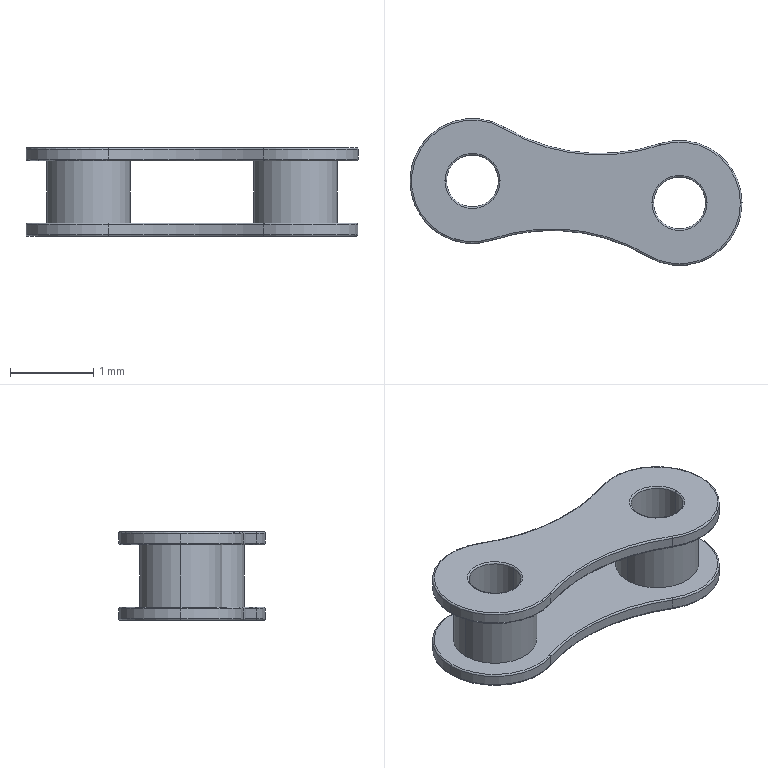Part | SolidWorks | features Scale 3, CombineBodies 1, Extrusion 1, Fillet 1, ICE 1, MirrorSolid 1 | 1 solid | 50 faces | box 3.986 x 1.764 x 1.063 mm | volume 1.997 mm3 | torus 28 | cylinder 18 | plane 4 | commonest cylinder face diameters 1.5 x6 0.625 x4 1 x4 4.5 x4
STEP:
#1=CARTESIAN_POINT('',(-79.03,0.9663,0.5313));
#2=VERTEX_POINT('',#1);
#3=CARTESIAN_POINT('',(-78.367,0.9663,0.5313));
#4=VERTEX_POINT('',#3);
#5=CARTESIAN_POINT('',(-78.699,0.9663,0.5313));
#6=DIRECTION('',(0.,0.,-1.));
#7=DIRECTION('',(1.,0.,0.));
#8=AXIS2_PLACEMENT_3D('',#5,#6,#7);
#9=CIRCLE('',#8,0.3313);
#10=EDGE_CURVE('',#2,#4,#9,.T.);
#11=ORIENTED_EDGE('',*,*,#10,.F.);
#12=CARTESIAN_POINT('',(-79.011,0.9663,0.5125));
#13=VERTEX_POINT('',#12);
#14=CARTESIAN_POINT('',(-79.03,0.9663,0.5125));
#15=DIRECTION('',(0.,1.,0.));
#16=DIRECTION('',(-1.,0.,0.));
#17=AXIS2_PLACEMENT_3D('',#14,#15,#16);
#18=CIRCLE('',#17,0.01875);
#19=EDGE_CURVE('',#2,#13,#18,.T.);
#20=ORIENTED_EDGE('',*,*,#19,.T.);
#21=CARTESIAN_POINT('',(-78.386,0.9663,0.5125));
#22=VERTEX_POINT('',#21);
#23=CARTESIAN_POINT('',(-78.699,0.9663,0.5125));
#24=DIRECTION('',(0.,0.,1.));
#25=DIRECTION('',(1.,0.,0.));
#26=AXIS2_PLACEMENT_3D('',#23,#24,#25);
#27=CIRCLE('',#26,0.3125);
#28=EDGE_CURVE('',#22,#13,#27,.T.);
#29=ORIENTED_EDGE('',*,*,#28,.F.);
#30=CARTESIAN_POINT('',(-78.367,0.9663,0.5125));
#31=DIRECTION('',(0.,-1.,0.));
#32=DIRECTION('',(0.,0.,-1.));
#33=AXIS2_PLACEMENT_3D('',#30,#31,#32);
#34=CIRCLE('',#33,0.01875);
#35=EDGE_CURVE('',#4,#22,#34,.T.);
#36=ORIENTED_EDGE('',*,*,#35,.F.);
#37=EDGE_LOOP('',(#11,#20,#29,#36));
#38=FACE_OUTER_BOUND('',#37,.T.);
#39=CARTESIAN_POINT('',(-78.699,0.9663,0.5125));
#40=DIRECTION('',(0.,0.,1.));
#41=DIRECTION('',(1.,0.,0.));
#42=AXIS2_PLACEMENT_3D('',#39,#40,#41);
#43=TOROIDAL_SURFACE('',#42,0.3312,0.01875);
#44=ADVANCED_FACE('',(#38),#43,.T.);
#45=CARTESIAN_POINT('',(-78.367,0.9663,-0.5312));
#46=VERTEX_POINT('',#45);
#47=CARTESIAN_POINT('',(-79.03,0.9663,-0.5312));
#48=VERTEX_POINT('',#47);
#49=CARTESIAN_POINT('',(-78.699,0.9663,-0.5312));
#50=DIRECTION('',(0.,0.,1.));
#51=DIRECTION('',(-1.,0.,0.));
#52=AXIS2_PLACEMENT_3D('',#49,#50,#51);
#53=CIRCLE('',#52,0.3313);
#54=EDGE_CURVE('',#46,#48,#53,.T.);
#55=ORIENTED_EDGE('',*,*,#54,.F.);
#56=CARTESIAN_POINT('',(-78.386,0.9663,-0.5125));
#57=VERTEX_POINT('',#56);
#58=CARTESIAN_POINT('',(-78.367,0.9663,-0.5125));
#59=DIRECTION('',(0.,1.,0.));
#60=DIRECTION('',(-1.,0.,0.));
#61=AXIS2_PLACEMENT_3D('',#58,#59,#60);
#62=CIRCLE('',#61,0.01875);
#63=EDGE_CURVE('',#46,#57,#62,.T.);
#64=ORIENTED_EDGE('',*,*,#63,.T.);
#65=CARTESIAN_POINT('',(-79.011,0.9663,-0.5125));
#66=VERTEX_POINT('',#65);
#67=CARTESIAN_POINT('',(-78.699,0.9663,-0.5125));
#68=DIRECTION('',(0.,0.,-1.));
#69=DIRECTION('',(-1.,0.,0.));
#70=AXIS2_PLACEMENT_3D('',#67,#68,#69);
#71=CIRCLE('',#70,0.3125);
#72=EDGE_CURVE('',#66,#57,#71,.T.);
#73=ORIENTED_EDGE('',*,*,#72,.F.);
#74=CARTESIAN_POINT('',(-79.03,0.9663,-0.5125));
#75=DIRECTION('',(0.,-1.,0.));
#76=DIRECTION('',(0.,0.,-1.));
#77=AXIS2_PLACEMENT_3D('',#74,#75,#76);
#78=CIRCLE('',#77,0.01875);
#79=EDGE_CURVE('',#48,#66,#78,.T.);
#80=ORIENTED_EDGE('',*,*,#79,.F.);
#81=EDGE_LOOP('',(#55,#64,#73,#80));
#82=FACE_OUTER_BOUND('',#81,.T.);
#83=CARTESIAN_POINT('',(-78.699,0.9663,-0.5125));
#84=DIRECTION('',(0.,0.,-1.));
#85=DIRECTION('',(-1.,0.,0.));
#86=AXIS2_PLACEMENT_3D('',#83,#84,#85);
#87=TOROIDAL_SURFACE('',#86,0.3312,0.01875);
#88=ADVANCED_FACE('',(#82),#87,.T.);
#89=CARTESIAN_POINT('',(-76.544,0.7018,0.5313));
#90=VERTEX_POINT('',#89);
#91=CARTESIAN_POINT('',(-75.881,0.7018,0.5313));
#92=VERTEX_POINT('',#91);
#93=CARTESIAN_POINT('',(-76.213,0.7018,0.5313));
#94=DIRECTION('',(0.,0.,-1.));
#95=DIRECTION('',(1.,0.,0.));
#96=AXIS2_PLACEMENT_3D('',#93,#94,#95);
#97=CIRCLE('',#96,0.3313);
#98=EDGE_CURVE('',#90,#92,#97,.T.);
#99=ORIENTED_EDGE('',*,*,#98,.F.);
#100=CARTESIAN_POINT('',(-76.525,0.7018,0.5125));
#101=VERTEX_POINT('',#100);
#102=CARTESIAN_POINT('',(-76.544,0.7018,0.5125));
#103=DIRECTION('',(0.,1.,0.));
#104=DIRECTION('',(-1.,0.,0.));
#105=AXIS2_PLACEMENT_3D('',#102,#103,#104);
#106=CIRCLE('',#105,0.01875);
#107=EDGE_CURVE('',#90,#101,#106,.T.);
#108=ORIENTED_EDGE('',*,*,#107,.T.);
#109=CARTESIAN_POINT('',(-75.9,0.7018,0.5125));
#110=VERTEX_POINT('',#109);
#111=CARTESIAN_POINT('',(-76.213,0.7018,0.5125));
#112=DIRECTION('',(0.,0.,1.));
#113=DIRECTION('',(1.,0.,0.));
#114=AXIS2_PLACEMENT_3D('',#111,#112,#113);
#115=CIRCLE('',#114,0.3125);
#116=EDGE_CURVE('',#110,#101,#115,.T.);
#117=ORIENTED_EDGE('',*,*,#116,.F.);
#118=CARTESIAN_POINT('',(-75.881,0.7018,0.5125));
#119=DIRECTION('',(0.,-1.,0.));
#120=DIRECTION('',(0.,0.,-1.));
#121=AXIS2_PLACEMENT_3D('',#118,#119,#120);
#122=CIRCLE('',#121,0.01875);
#123=EDGE_CURVE('',#92,#110,#122,.T.);
#124=ORIENTED_EDGE('',*,*,#123,.F.);
#125=EDGE_LOOP('',(#99,#108,#117,#124));
#126=FACE_OUTER_BOUND('',#125,.T.);
#127=CARTESIAN_POINT('',(-76.213,0.7018,0.5125));
#128=DIRECTION('',(0.,0.,1.));
#129=DIRECTION('',(1.,0.,0.));
#130=AXIS2_PLACEMENT_3D('',#127,#128,#129);
#131=TOROIDAL_SURFACE('',#130,0.3312,0.01875);
#132=ADVANCED_FACE('',(#126),#131,.T.);
#133=CARTESIAN_POINT('',(-75.881,0.7018,-0.5312));
#134=VERTEX_POINT('',#133);
#135=CARTESIAN_POINT('',(-76.544,0.7018,-0.5312));
#136=VERTEX_POINT('',#135);
#137=CARTESIAN_POINT('',(-76.213,0.7018,-0.5312));
#138=DIRECTION('',(0.,0.,1.));
#139=DIRECTION('',(-1.,0.,0.));
#140=AXIS2_PLACEMENT_3D('',#137,#138,#139);
#141=CIRCLE('',#140,0.3313);
#142=EDGE_CURVE('',#134,#136,#141,.T.);
#143=ORIENTED_EDGE('',*,*,#142,.F.);
#144=CARTESIAN_POINT('',(-75.9,0.7018,-0.5125));
#145=VERTEX_POINT('',#144);
#146=CARTESIAN_POINT('',(-75.881,0.7018,-0.5125));
#147=DIRECTION('',(0.,1.,0.));
#148=DIRECTION('',(-1.,0.,0.));
#149=AXIS2_PLACEMENT_3D('',#146,#147,#148);
#150=CIRCLE('',#149,0.01875);
#151=EDGE_CURVE('',#134,#145,#150,.T.);
#152=ORIENTED_EDGE('',*,*,#151,.T.);
#153=CARTESIAN_POINT('',(-76.525,0.7018,-0.5125));
#154=VERTEX_POINT('',#153);
#155=CARTESIAN_POINT('',(-76.213,0.7018,-0.5125));
#156=DIRECTION('',(0.,0.,-1.));
#157=DIRECTION('',(-1.,0.,0.));
#158=AXIS2_PLACEMENT_3D('',#155,#156,#157);
#159=CIRCLE('',#158,0.3125);
#160=EDGE_CURVE('',#154,#145,#159,.T.);
#161=ORIENTED_EDGE('',*,*,#160,.F.);
#162=CARTESIAN_POINT('',(-76.544,0.7018,-0.5125));
#163=DIRECTION('',(0.,-1.,0.));
#164=DIRECTION('',(0.,0.,-1.));
#165=AXIS2_PLACEMENT_3D('',#162,#163,#164);
#166=CIRCLE('',#165,0.01875);
#167=EDGE_CURVE('',#136,#154,#166,.T.);
#168=ORIENTED_EDGE('',*,*,#167,.F.);
#169=EDGE_LOOP('',(#143,#152,#161,#168));
#170=FACE_OUTER_BOUND('',#169,.T.);
#171=CARTESIAN_POINT('',(-76.213,0.7018,-0.5125));
#172=DIRECTION('',(0.,0.,-1.));
#173=DIRECTION('',(-1.,0.,0.));
#174=AXIS2_PLACEMENT_3D('',#171,#172,#173);
#175=TOROIDAL_SURFACE('',#174,0.3312,0.01875);
#176=ADVANCED_FACE('',(#170),#175,.T.);
#177=CARTESIAN_POINT('',(-75.481,0.7018,0.375));
#178=VERTEX_POINT('',#177);
#179=CARTESIAN_POINT('',(-76.586,0.07305,0.375));
#180=VERTEX_POINT('',#179);
#181=CARTESIAN_POINT('',(-76.213,0.7018,0.375));
#182=DIRECTION('',(0.,0.,-1.));
#183=DIRECTION('',(1.,0.,0.));
#184=AXIS2_PLACEMENT_3D('',#181,#182,#183);
#185=CIRCLE('',#184,0.7313);
#186=EDGE_CURVE('',#178,#180,#185,.T.);
#187=ORIENTED_EDGE('',*,*,#186,.F.);
#188=CARTESIAN_POINT('',(-75.463,0.7018,0.3938));
#189=VERTEX_POINT('',#188);
#190=CARTESIAN_POINT('',(-75.481,0.7018,0.3938));
#191=DIRECTION('',(0.,-1.,0.));
#192=DIRECTION('',(0.,0.,-1.));
#193=AXIS2_PLACEMENT_3D('',#190,#191,#192);
#194=CIRCLE('',#193,0.01875);
#195=EDGE_CURVE('',#178,#189,#194,.T.);
#196=ORIENTED_EDGE('',*,*,#195,.T.);
#197=CARTESIAN_POINT('',(-76.596,0.05692,0.3938));
#198=VERTEX_POINT('',#197);
#199=CARTESIAN_POINT('',(-76.213,0.7018,0.3938));
#200=DIRECTION('',(0.,0.,1.));
#201=DIRECTION('',(1.,0.,0.));
#202=AXIS2_PLACEMENT_3D('',#199,#200,#201);
#203=CIRCLE('',#202,0.75);
#204=EDGE_CURVE('',#198,#189,#203,.T.);
#205=ORIENTED_EDGE('',*,*,#204,.F.);
#206=CARTESIAN_POINT('',(-76.586,0.07305,0.3938));
#207=DIRECTION('',(0.8599,-0.5105,0.));
#208=DIRECTION('',(0.5105,0.8599,0.));
#209=AXIS2_PLACEMENT_3D('',#206,#207,#208);
#210=CIRCLE('',#209,0.01875);
#211=EDGE_CURVE('',#198,#180,#210,.T.);
#212=ORIENTED_EDGE('',*,*,#211,.T.);
#213=EDGE_LOOP('',(#187,#196,#205,#212));
#214=FACE_OUTER_BOUND('',#213,.T.);
#215=CARTESIAN_POINT('',(-76.213,0.7018,0.3938));
#216=DIRECTION('',(0.,0.,1.));
#217=DIRECTION('',(1.,0.,0.));
#218=AXIS2_PLACEMENT_3D('',#215,#216,#217);
#219=TOROIDAL_SURFACE('',#218,0.7313,0.01875);
#220=ADVANCED_FACE('',(#214),#219,.T.);
#221=CARTESIAN_POINT('',(-75.463,0.7018,0.5125));
#222=VERTEX_POINT('',#221);
#223=CARTESIAN_POINT('',(-76.596,0.05692,0.5125));
#224=VERTEX_POINT('',#223);
#225=CARTESIAN_POINT('',(-76.213,0.7018,0.5125));
#226=DIRECTION('',(0.,0.,-1.));
#227=DIRECTION('',(1.,0.,0.));
#228=AXIS2_PLACEMENT_3D('',#225,#226,#227);
#229=CIRCLE('',#228,0.75);
#230=EDGE_CURVE('',#222,#224,#229,.T.);
#231=ORIENTED_EDGE('',*,*,#230,.F.);
#232=CARTESIAN_POINT('',(-75.481,0.7018,0.5313));
#233=VERTEX_POINT('',#232);
#234=CARTESIAN_POINT('',(-75.481,0.7018,0.5125));
#235=DIRECTION('',(0.,-1.,0.));
#236=DIRECTION('',(0.,0.,-1.));
#237=AXIS2_PLACEMENT_3D('',#234,#235,#236);
#238=CIRCLE('',#237,0.01875);
#239=EDGE_CURVE('',#222,#233,#238,.T.);
#240=ORIENTED_EDGE('',*,*,#239,.T.);
#241=CARTESIAN_POINT('',(-76.586,0.07305,0.5313));
#242=VERTEX_POINT('',#241);
#243=CARTESIAN_POINT('',(-76.213,0.7018,0.5313));
#244=DIRECTION('',(0.,0.,1.));
#245=DIRECTION('',(1.,0.,0.));
#246=AXIS2_PLACEMENT_3D('',#243,#244,#245);
#247=CIRCLE('',#246,0.7313);
#248=EDGE_CURVE('',#242,#233,#247,.T.);
#249=ORIENTED_EDGE('',*,*,#248,.F.);
#250=CARTESIAN_POINT('',(-76.586,0.07305,0.5125));
#251=DIRECTION('',(0.8599,-0.5105,0.));
#252=DIRECTION('',(0.5105,0.8599,0.));
#253=AXIS2_PLACEMENT_3D('',#250,#251,#252);
#254=CIRCLE('',#253,0.01875);
#255=EDGE_CURVE('',#242,#224,#254,.T.);
#256=ORIENTED_EDGE('',*,*,#255,.T.);
#257=EDGE_LOOP('',(#231,#240,#249,#256));
#258=FACE_OUTER_BOUND('',#257,.T.);
#259=CARTESIAN_POINT('',(-76.213,0.7018,0.5125));
#260=DIRECTION('',(0.,0.,1.));
#261=DIRECTION('',(1.,0.,0.));
#262=AXIS2_PLACEMENT_3D('',#259,#260,#261);
#263=TOROIDAL_SURFACE('',#262,0.7313,0.01875);
#264=ADVANCED_FACE('',(#258),#263,.T.);
#265=CARTESIAN_POINT('',(-79.43,0.9663,-0.375));
#266=VERTEX_POINT('',#265);
#267=CARTESIAN_POINT('',(-78.466,0.273,-0.375));
#268=VERTEX_POINT('',#267);
#269=CARTESIAN_POINT('',(-78.699,0.9663,-0.375));
#270=DIRECTION('',(0.,0.,1.));
#271=DIRECTION('',(-1.,0.,0.));
#272=AXIS2_PLACEMENT_3D('',#269,#270,#271);
#273=CIRCLE('',#272,0.7313);
#274=EDGE_CURVE('',#266,#268,#273,.T.);
#275=ORIENTED_EDGE('',*,*,#274,.F.);
#276=CARTESIAN_POINT('',(-79.449,0.9663,-0.3937));
#277=VERTEX_POINT('',#276);
#278=CARTESIAN_POINT('',(-79.43,0.9663,-0.3937));
#279=DIRECTION('',(0.,-1.,0.));
#280=DIRECTION('',(0.,0.,-1.));
#281=AXIS2_PLACEMENT_3D('',#278,#279,#280);
#282=CIRCLE('',#281,0.01875);
#283=EDGE_CURVE('',#266,#277,#282,.T.);
#284=ORIENTED_EDGE('',*,*,#283,.T.);
#285=CARTESIAN_POINT('',(-78.46,0.2552,-0.3937));
#286=VERTEX_POINT('',#285);
#287=CARTESIAN_POINT('',(-78.699,0.9663,-0.3937));
#288=DIRECTION('',(0.,0.,-1.));
#289=DIRECTION('',(-1.,0.,0.));
#290=AXIS2_PLACEMENT_3D('',#287,#288,#289);
#291=CIRCLE('',#290,0.75);
#292=EDGE_CURVE('',#286,#277,#291,.T.);
#293=ORIENTED_EDGE('',*,*,#292,.F.);
#294=CARTESIAN_POINT('',(-78.466,0.273,-0.3937));
#295=DIRECTION('',(0.948,0.3182,0.));
#296=DIRECTION('',(-0.3182,0.948,0.));
#297=AXIS2_PLACEMENT_3D('',#294,#295,#296);
#298=CIRCLE('',#297,0.01875);
#299=EDGE_CURVE('',#268,#286,#298,.T.);
#300=ORIENTED_EDGE('',*,*,#299,.F.);
#301=EDGE_LOOP('',(#275,#284,#293,#300));
#302=FACE_OUTER_BOUND('',#301,.T.);
#303=CARTESIAN_POINT('',(-78.699,0.9663,-0.3937));
#304=DIRECTION('',(0.,0.,-1.));
#305=DIRECTION('',(-1.,0.,0.));
#306=AXIS2_PLACEMENT_3D('',#303,#304,#305);
#307=TOROIDAL_SURFACE('',#306,0.7313,0.01875);
#308=ADVANCED_FACE('',(#302),#307,.T.);
#309=CARTESIAN_POINT('',(-79.449,0.9663,-0.5125));
#310=VERTEX_POINT('',#309);
#311=CARTESIAN_POINT('',(-78.46,0.2552,-0.5125));
#312=VERTEX_POINT('',#311);
#313=CARTESIAN_POINT('',(-78.699,0.9663,-0.5125));
#314=DIRECTION('',(0.,0.,1.));
#315=DIRECTION('',(-1.,0.,0.));
#316=AXIS2_PLACEMENT_3D('',#313,#314,#315);
#317=CIRCLE('',#316,0.75);
#318=EDGE_CURVE('',#310,#312,#317,.T.);
#319=ORIENTED_EDGE('',*,*,#318,.F.);
#320=CARTESIAN_POINT('',(-79.43,0.9663,-0.5312));
#321=VERTEX_POINT('',#320);
#322=CARTESIAN_POINT('',(-79.43,0.9663,-0.5125));
#323=DIRECTION('',(0.,-1.,0.));
#324=DIRECTION('',(0.,0.,-1.));
#325=AXIS2_PLACEMENT_3D('',#322,#323,#324);
#326=CIRCLE('',#325,0.01875);
#327=EDGE_CURVE('',#310,#321,#326,.T.);
#328=ORIENTED_EDGE('',*,*,#327,.T.);
#329=CARTESIAN_POINT('',(-78.466,0.273,-0.5312));
#330=VERTEX_POINT('',#329);
#331=CARTESIAN_POINT('',(-78.699,0.9663,-0.5312));
#332=DIRECTION('',(0.,0.,-1.));
#333=DIRECTION('',(-1.,0.,0.));
#334=AXIS2_PLACEMENT_3D('',#331,#332,#333);
#335=CIRCLE('',#334,0.7313);
#336=EDGE_CURVE('',#330,#321,#335,.T.);
#337=ORIENTED_EDGE('',*,*,#336,.F.);
#338=CARTESIAN_POINT('',(-78.466,0.273,-0.5125));
#339=DIRECTION('',(0.948,0.3182,0.));
#340=DIRECTION('',(-0.3182,0.948,0.));
#341=AXIS2_PLACEMENT_3D('',#338,#339,#340);
#342=CIRCLE('',#341,0.01875);
#343=EDGE_CURVE('',#312,#330,#342,.T.);
#344=ORIENTED_EDGE('',*,*,#343,.F.);
#345=EDGE_LOOP('',(#319,#328,#337,#344));
#346=FACE_OUTER_BOUND('',#345,.T.);
#347=CARTESIAN_POINT('',(-78.699,0.9663,-0.5125));
#348=DIRECTION('',(0.,0.,-1.));
#349=DIRECTION('',(-1.,0.,0.));
#350=AXIS2_PLACEMENT_3D('',#347,#348,#349);
#351=TOROIDAL_SURFACE('',#350,0.7313,0.01875);
#352=ADVANCED_FACE('',(#346),#351,.T.);
#353=CARTESIAN_POINT('',(-75.713,0.7018,-0.375));
#354=VERTEX_POINT('',#353);
#355=CARTESIAN_POINT('',(-76.713,0.7018,-0.375));
#356=VERTEX_POINT('',#355);
#357=CARTESIAN_POINT('',(-76.213,0.7018,-0.375));
#358=DIRECTION('',(0.,0.,1.));
#359=DIRECTION('',(1.,0.,0.));
#360=AXIS2_PLACEMENT_3D('',#357,#358,#359);
#361=CIRCLE('',#360,0.5);
#362=EDGE_CURVE('',#354,#356,#361,.T.);
#363=ORIENTED_EDGE('',*,*,#362,.T.);
#364=CARTESIAN_POINT('',(-76.713,0.7018,0.375));
#365=VERTEX_POINT('',#364);
#366=CARTESIAN_POINT('',(-76.713,0.7018,-0.375));
#367=DIRECTION('',(0.,0.,1.));
#368=VECTOR('',#367,1000.);
#369=LINE('',#366,#368);
#370=EDGE_CURVE('',#356,#365,#369,.T.);
#371=ORIENTED_EDGE('',*,*,#370,.T.);
#372=CARTESIAN_POINT('',(-75.713,0.7018,0.375));
#373=VERTEX_POINT('',#372);
#374=CARTESIAN_POINT('',(-76.213,0.7018,0.375));
#375=DIRECTION('',(0.,0.,1.));
#376=DIRECTION('',(1.,0.,0.));
#377=AXIS2_PLACEMENT_3D('',#374,#375,#376);
#378=CIRCLE('',#377,0.5);
#379=EDGE_CURVE('',#373,#365,#378,.T.);
#380=ORIENTED_EDGE('',*,*,#379,.F.);
#381=CARTESIAN_POINT('',(-75.713,0.7018,-0.375));
#382=DIRECTION('',(0.,0.,1.));
#383=VECTOR('',#382,1000.);
#384=LINE('',#381,#383);
#385=EDGE_CURVE('',#354,#373,#384,.T.);
#386=ORIENTED_EDGE('',*,*,#385,.F.);
#387=EDGE_LOOP('',(#363,#371,#380,#386));
#388=FACE_OUTER_BOUND('',#387,.T.);
#389=CARTESIAN_POINT('',(-76.213,0.7018,-0.375));
#390=DIRECTION('',(0.,0.,1.));
#391=DIRECTION('',(1.,0.,0.));
#392=AXIS2_PLACEMENT_3D('',#389,#390,#391);
#393=CYLINDRICAL_SURFACE('',#392,0.5);
#394=ADVANCED_FACE('',(#388),#393,.T.);
#395=CARTESIAN_POINT('',(-78.316,1.611,-0.5125));
#396=VERTEX_POINT('',#395);
#397=CARTESIAN_POINT('',(-78.699,0.9663,-0.5125));
#398=DIRECTION('',(0.,0.,1.));
#399=DIRECTION('',(-1.,0.,0.));
#400=AXIS2_PLACEMENT_3D('',#397,#398,#399);
#401=CIRCLE('',#400,0.75);
#402=EDGE_CURVE('',#396,#310,#401,.T.);
#403=ORIENTED_EDGE('',*,*,#402,.T.);
#404=CARTESIAN_POINT('',(-79.449,0.9663,-0.5312));
#405=DIRECTION('',(0.,0.,1.));
#406=VECTOR('',#405,1000.);
#407=LINE('',#404,#406);
#408=EDGE_CURVE('',#310,#277,#407,.T.);
#409=ORIENTED_EDGE('',*,*,#408,.T.);
#410=CARTESIAN_POINT('',(-78.316,1.611,-0.3937));
#411=VERTEX_POINT('',#410);
#412=CARTESIAN_POINT('',(-78.699,0.9663,-0.3937));
#413=DIRECTION('',(0.,0.,-1.));
#414=DIRECTION('',(-1.,0.,0.));
#415=AXIS2_PLACEMENT_3D('',#412,#413,#414);
#416=CIRCLE('',#415,0.75);
#417=EDGE_CURVE('',#277,#411,#416,.T.);
#418=ORIENTED_EDGE('',*,*,#417,.T.);
#419=CARTESIAN_POINT('',(-78.316,1.611,-0.5312));
#420=DIRECTION('',(0.,0.,1.));
#421=VECTOR('',#420,1000.);
#422=LINE('',#419,#421);
#423=EDGE_CURVE('',#396,#411,#422,.T.);
#424=ORIENTED_EDGE('',*,*,#423,.F.);
#425=EDGE_LOOP('',(#403,#409,#418,#424));
#426=FACE_OUTER_BOUND('',#425,.T.);
#427=CARTESIAN_POINT('',(-78.699,0.9663,-0.5312));
#428=DIRECTION('',(0.,0.,1.));
#429=DIRECTION('',(-1.,0.,0.));
#430=AXIS2_PLACEMENT_3D('',#427,#428,#429);
#431=CYLINDRICAL_SURFACE('',#430,0.75);
#432=ADVANCED_FACE('',(#426),#431,.T.);
#433=CARTESIAN_POINT('',(-78.199,0.9663,-0.375));
#434=VERTEX_POINT('',#433);
#435=CARTESIAN_POINT('',(-79.199,0.9663,-0.375));
#436=VERTEX_POINT('',#435);
#437=CARTESIAN_POINT('',(-78.699,0.9663,-0.375));
#438=DIRECTION('',(0.,0.,1.));
#439=DIRECTION('',(-1.,0.,0.));
#440=AXIS2_PLACEMENT_3D('',#437,#438,#439);
#441=CIRCLE('',#440,0.5);
#442=EDGE_CURVE('',#434,#436,#441,.T.);
#443=ORIENTED_EDGE('',*,*,#442,.T.);
#444=CARTESIAN_POINT('',(-79.199,0.9663,0.375));
#445=VERTEX_POINT('',#444);
#446=CARTESIAN_POINT('',(-79.199,0.9663,-0.375));
#447=DIRECTION('',(0.,0.,1.));
#448=VECTOR('',#447,1000.);
#449=LINE('',#446,#448);
#450=EDGE_CURVE('',#436,#445,#449,.T.);
#451=ORIENTED_EDGE('',*,*,#450,.T.);
#452=CARTESIAN_POINT('',(-78.199,0.9663,0.375));
#453=VERTEX_POINT('',#452);
#454=CARTESIAN_POINT('',(-78.699,0.9663,0.375));
#455=DIRECTION('',(0.,0.,1.));
#456=DIRECTION('',(1.,0.,0.));
#457=AXIS2_PLACEMENT_3D('',#454,#455,#456);
#458=CIRCLE('',#457,0.5);
#459=EDGE_CURVE('',#453,#445,#458,.T.);
#460=ORIENTED_EDGE('',*,*,#459,.F.);
#461=CARTESIAN_POINT('',(-78.199,0.9663,-0.375));
#462=DIRECTION('',(0.,0.,1.));
#463=VECTOR('',#462,1000.);
#464=LINE('',#461,#463);
#465=EDGE_CURVE('',#434,#453,#464,.T.);
#466=ORIENTED_EDGE('',*,*,#465,.F.);
#467=EDGE_LOOP('',(#443,#451,#460,#466));
#468=FACE_OUTER_BOUND('',#467,.T.);
#469=CARTESIAN_POINT('',(-78.699,0.9663,-0.375));
#470=DIRECTION('',(0.,0.,1.));
#471=DIRECTION('',(1.,0.,0.));
#472=AXIS2_PLACEMENT_3D('',#469,#470,#471);
#473=CYLINDRICAL_SURFACE('',#472,0.5);
#474=ADVANCED_FACE('',(#468),#473,.T.);
#475=CARTESIAN_POINT('',(-78.699,0.9663,0.5125));
#476=DIRECTION('',(0.,0.,1.));
#477=DIRECTION('',(1.,0.,0.));
#478=AXIS2_PLACEMENT_3D('',#475,#476,#477);
#479=CIRCLE('',#478,0.3125);
#480=EDGE_CURVE('',#13,#22,#479,.T.);
#481=ORIENTED_EDGE('',*,*,#480,.T.);
#482=CARTESIAN_POINT('',(-78.386,0.9663,0.5313));
#483=DIRECTION('',(0.,0.,-1.));
#484=VECTOR('',#483,1000.);
#485=LINE('',#482,#484);
#486=EDGE_CURVE('',#22,#57,#485,.T.);
#487=ORIENTED_EDGE('',*,*,#486,.T.);
#488=CARTESIAN_POINT('',(-78.699,0.9663,-0.5125));
#489=DIRECTION('',(0.,0.,-1.));
#490=DIRECTION('',(-1.,0.,0.));
#491=AXIS2_PLACEMENT_3D('',#488,#489,#490);
#492=CIRCLE('',#491,0.3125);
#493=EDGE_CURVE('',#57,#66,#492,.T.);
#494=ORIENTED_EDGE('',*,*,#493,.T.);
#495=CARTESIAN_POINT('',(-79.011,0.9663,0.5313));
#496=DIRECTION('',(0.,0.,-1.));
#497=VECTOR('',#496,1000.);
#498=LINE('',#495,#497);
#499=EDGE_CURVE('',#13,#66,#498,.T.);
#500=ORIENTED_EDGE('',*,*,#499,.F.);
#501=EDGE_LOOP('',(#481,#487,#494,#500));
#502=FACE_OUTER_BOUND('',#501,.T.);
#503=CARTESIAN_POINT('',(-78.699,0.9663,0.5313));
#504=DIRECTION('',(0.,0.,-1.));
#505=DIRECTION('',(-1.,0.,0.));
#506=AXIS2_PLACEMENT_3D('',#503,#504,#505);
#507=CYLINDRICAL_SURFACE('',#506,0.3125);
#508=ADVANCED_FACE('',(#502),#507,.F.);
#509=CARTESIAN_POINT('',(-76.213,0.7018,0.5125));
#510=DIRECTION('',(0.,0.,1.));
#511=DIRECTION('',(1.,0.,0.));
#512=AXIS2_PLACEMENT_3D('',#509,#510,#511);
#513=CIRCLE('',#512,0.3125);
#514=EDGE_CURVE('',#101,#110,#513,.T.);
#515=ORIENTED_EDGE('',*,*,#514,.T.);
#516=CARTESIAN_POINT('',(-75.9,0.7018,0.5313));
#517=DIRECTION('',(0.,0.,-1.));
#518=VECTOR('',#517,1000.);
#519=LINE('',#516,#518);
#520=EDGE_CURVE('',#110,#145,#519,.T.);
#521=ORIENTED_EDGE('',*,*,#520,.T.);
#522=CARTESIAN_POINT('',(-76.213,0.7018,-0.5125));
#523=DIRECTION('',(0.,0.,-1.));
#524=DIRECTION('',(-1.,0.,0.));
#525=AXIS2_PLACEMENT_3D('',#522,#523,#524);
#526=CIRCLE('',#525,0.3125);
#527=EDGE_CURVE('',#145,#154,#526,.T.);
#528=ORIENTED_EDGE('',*,*,#527,.T.);
#529=CARTESIAN_POINT('',(-76.525,0.7018,0.5313));
#530=DIRECTION('',(0.,0.,-1.));
#531=VECTOR('',#530,1000.);
#532=LINE('',#529,#531);
#533=EDGE_CURVE('',#101,#154,#532,.T.);
#534=ORIENTED_EDGE('',*,*,#533,.F.);
#535=EDGE_LOOP('',(#515,#521,#528,#534));
#536=FACE_OUTER_BOUND('',#535,.T.);
#537=CARTESIAN_POINT('',(-76.213,0.7018,0.5313));
#538=DIRECTION('',(0.,0.,-1.));
#539=DIRECTION('',(-1.,0.,0.));
#540=AXIS2_PLACEMENT_3D('',#537,#538,#539);
#541=CYLINDRICAL_SURFACE('',#540,0.3125);
#542=ADVANCED_FACE('',(#536),#541,.F.);
#543=CARTESIAN_POINT('',(-78.46,0.2552,0.5125));
#544=VERTEX_POINT('',#543);
#545=CARTESIAN_POINT('',(-79.449,0.9663,0.5125));
#546=VERTEX_POINT('',#545);
#547=CARTESIAN_POINT('',(-78.699,0.9663,0.5125));
#548=DIRECTION('',(0.,0.,-1.));
#549=DIRECTION('',(1.,0.,0.));
#550=AXIS2_PLACEMENT_3D('',#547,#548,#549);
#551=CIRCLE('',#550,0.75);
#552=EDGE_CURVE('',#544,#546,#551,.T.);
#553=ORIENTED_EDGE('',*,*,#552,.T.);
#554=CARTESIAN_POINT('',(-79.449,0.9663,0.3938));
#555=VERTEX_POINT('',#554);
#556=CARTESIAN_POINT('',(-79.449,0.9663,0.5313));
#557=DIRECTION('',(0.,0.,-1.));
#558=VECTOR('',#557,1000.);
#559=LINE('',#556,#558);
#560=EDGE_CURVE('',#546,#555,#559,.T.);
#561=ORIENTED_EDGE('',*,*,#560,.T.);
#562=CARTESIAN_POINT('',(-78.46,0.2552,0.3938));
#563=VERTEX_POINT('',#562);
#564=CARTESIAN_POINT('',(-78.699,0.9663,0.3938));
#565=DIRECTION('',(0.,0.,1.));
#566=DIRECTION('',(1.,0.,0.));
#567=AXIS2_PLACEMENT_3D('',#564,#565,#566);
#568=CIRCLE('',#567,0.75);
#569=EDGE_CURVE('',#555,#563,#568,.T.);
#570=ORIENTED_EDGE('',*,*,#569,.T.);
#571=CARTESIAN_POINT('',(-78.46,0.2552,0.5313));
#572=DIRECTION('',(0.,0.,-1.));
#573=VECTOR('',#572,1000.);
#574=LINE('',#571,#573);
#575=EDGE_CURVE('',#544,#563,#574,.T.);
#576=ORIENTED_EDGE('',*,*,#575,.F.);
#577=EDGE_LOOP('',(#553,#561,#570,#576));
#578=FACE_OUTER_BOUND('',#577,.T.);
#579=CARTESIAN_POINT('',(-78.699,0.9663,0.5313));
#580=DIRECTION('',(0.,0.,-1.));
#581=DIRECTION('',(-1.,0.,0.));
#582=AXIS2_PLACEMENT_3D('',#579,#580,#581);
#583=CYLINDRICAL_SURFACE('',#582,0.75);
#584=ADVANCED_FACE('',(#578),#583,.T.);
#585=CARTESIAN_POINT('',(-76.213,0.7018,0.5313));
#586=DIRECTION('',(0.,0.,-1.));
#587=DIRECTION('',(1.,0.,0.));
#588=AXIS2_PLACEMENT_3D('',#585,#586,#587);
#589=CIRCLE('',#588,0.3313);
#590=EDGE_CURVE('',#92,#90,#589,.T.);
#591=ORIENTED_EDGE('',*,*,#590,.T.);
#592=ORIENTED_EDGE('',*,*,#98,.T.);
#593=EDGE_LOOP('',(#591,#592));
#594=FACE_BOUND('',#593,.T.);
#595=CARTESIAN_POINT('',(-78.699,0.9663,0.5313));
#596=DIRECTION('',(0.,0.,-1.));
#597=DIRECTION('',(1.,0.,0.));
#598=AXIS2_PLACEMENT_3D('',#595,#596,#597);
#599=CIRCLE('',#598,0.3313);
#600=EDGE_CURVE('',#4,#2,#599,.T.);
#601=ORIENTED_EDGE('',*,*,#600,.T.);
#602=ORIENTED_EDGE('',*,*,#10,.T.);
#603=EDGE_LOOP('',(#601,#602));
#604=FACE_BOUND('',#603,.T.);
#605=CARTESIAN_POINT('',(-78.466,0.273,0.5313));
#606=VERTEX_POINT('',#605);
#607=CARTESIAN_POINT('',(-77.744,-1.878,0.5313));
#608=DIRECTION('',(0.,0.,-1.));
#609=DIRECTION('',(1.,0.,0.));
#610=AXIS2_PLACEMENT_3D('',#607,#608,#609);
#611=CIRCLE('',#610,2.269);
#612=EDGE_CURVE('',#606,#242,#611,.T.);
#613=ORIENTED_EDGE('',*,*,#612,.T.);
#614=ORIENTED_EDGE('',*,*,#248,.T.);
#615=CARTESIAN_POINT('',(-76.445,1.395,0.5313));
#616=VERTEX_POINT('',#615);
#617=CARTESIAN_POINT('',(-76.213,0.7018,0.5313));
#618=DIRECTION('',(0.,0.,1.));
#619=DIRECTION('',(1.,0.,0.));
#620=AXIS2_PLACEMENT_3D('',#617,#618,#619);
#621=CIRCLE('',#620,0.7313);
#622=EDGE_CURVE('',#233,#616,#621,.T.);
#623=ORIENTED_EDGE('',*,*,#622,.T.);
#624=CARTESIAN_POINT('',(-78.325,1.595,0.5313));
#625=VERTEX_POINT('',#624);
#626=CARTESIAN_POINT('',(-77.167,3.546,0.5313));
#627=DIRECTION('',(0.,0.,-1.));
#628=DIRECTION('',(1.,0.,0.));
#629=AXIS2_PLACEMENT_3D('',#626,#627,#628);
#630=CIRCLE('',#629,2.269);
#631=EDGE_CURVE('',#616,#625,#630,.T.);
#632=ORIENTED_EDGE('',*,*,#631,.T.);
#633=CARTESIAN_POINT('',(-78.699,0.9663,0.5313));
#634=DIRECTION('',(0.,0.,1.));
#635=DIRECTION('',(1.,0.,0.));
#636=AXIS2_PLACEMENT_3D('',#633,#634,#635);
#637=CIRCLE('',#636,0.7313);
#638=EDGE_CURVE('',#625,#606,#637,.T.);
#639=ORIENTED_EDGE('',*,*,#638,.T.);
#640=EDGE_LOOP('',(#613,#614,#623,#632,#639));
#641=FACE_OUTER_BOUND('',#640,.T.);
#642=CARTESIAN_POINT('',(-78.221,-0.4558,0.5313));
#643=DIRECTION('',(0.,0.,1.));
#644=DIRECTION('',(1.,0.,0.));
#645=AXIS2_PLACEMENT_3D('',#642,#643,#644);
#646=PLANE('',#645);
#647=ADVANCED_FACE('',(#594,#604,#641),#646,.T.);
#648=CARTESIAN_POINT('',(-78.325,1.595,0.375));
#649=VERTEX_POINT('',#648);
#650=CARTESIAN_POINT('',(-76.445,1.395,0.375));
#651=VERTEX_POINT('',#650);
#652=CARTESIAN_POINT('',(-77.167,3.546,0.375));
#653=DIRECTION('',(0.,0.,1.));
#654=DIRECTION('',(1.,0.,0.));
#655=AXIS2_PLACEMENT_3D('',#652,#653,#654);
#656=CIRCLE('',#655,2.269);
#657=EDGE_CURVE('',#649,#651,#656,.T.);
#658=ORIENTED_EDGE('',*,*,#657,.T.);
#659=CARTESIAN_POINT('',(-76.213,0.7018,0.375));
#660=DIRECTION('',(0.,0.,-1.));
#661=DIRECTION('',(1.,0.,0.));
#662=AXIS2_PLACEMENT_3D('',#659,#660,#661);
#663=CIRCLE('',#662,0.7313);
#664=EDGE_CURVE('',#651,#178,#663,.T.);
#665=ORIENTED_EDGE('',*,*,#664,.T.);
#666=ORIENTED_EDGE('',*,*,#186,.T.);
#667=CARTESIAN_POINT('',(-78.466,0.273,0.375));
#668=VERTEX_POINT('',#667);
#669=CARTESIAN_POINT('',(-77.744,-1.878,0.375));
#670=DIRECTION('',(0.,0.,1.));
#671=DIRECTION('',(1.,0.,0.));
#672=AXIS2_PLACEMENT_3D('',#669,#670,#671);
#673=CIRCLE('',#672,2.269);
#674=EDGE_CURVE('',#180,#668,#673,.T.);
#675=ORIENTED_EDGE('',*,*,#674,.T.);
#676=CARTESIAN_POINT('',(-78.699,0.9663,0.375));
#677=DIRECTION('',(0.,0.,-1.));
#678=DIRECTION('',(1.,0.,0.));
#679=AXIS2_PLACEMENT_3D('',#676,#677,#678);
#680=CIRCLE('',#679,0.7313);
#681=EDGE_CURVE('',#668,#649,#680,.T.);
#682=ORIENTED_EDGE('',*,*,#681,.T.);
#683=EDGE_LOOP('',(#658,#665,#666,#675,#682));
#684=FACE_OUTER_BOUND('',#683,.T.);
#685=ORIENTED_EDGE('',*,*,#459,.T.);
#686=CARTESIAN_POINT('',(-78.699,0.9663,0.375));
#687=DIRECTION('',(0.,0.,1.));
#688=DIRECTION('',(1.,0.,0.));
#689=AXIS2_PLACEMENT_3D('',#686,#687,#688);
#690=CIRCLE('',#689,0.5);
#691=EDGE_CURVE('',#445,#453,#690,.T.);
#692=ORIENTED_EDGE('',*,*,#691,.T.);
#693=EDGE_LOOP('',(#685,#692));
#694=FACE_BOUND('',#693,.T.);
#695=ORIENTED_EDGE('',*,*,#379,.T.);
#696=CARTESIAN_POINT('',(-76.213,0.7018,0.375));
#697=DIRECTION('',(0.,0.,1.));
#698=DIRECTION('',(1.,0.,0.));
#699=AXIS2_PLACEMENT_3D('',#696,#697,#698);
#700=CIRCLE('',#699,0.5);
#701=EDGE_CURVE('',#365,#373,#700,.T.);
#702=ORIENTED_EDGE('',*,*,#701,.T.);
#703=EDGE_LOOP('',(#695,#702));
#704=FACE_BOUND('',#703,.T.);
#705=CARTESIAN_POINT('',(-78.221,-0.4558,0.375));
#706=DIRECTION('',(0.,0.,1.));
#707=DIRECTION('',(1.,0.,0.));
#708=AXIS2_PLACEMENT_3D('',#705,#706,#707);
#709=PLANE('',#708);
#710=ADVANCED_FACE('',(#684,#694,#704),#709,.F.);
#711=CARTESIAN_POINT('',(-76.596,0.05692,0.5313));
#712=DIRECTION('',(0.,0.,-1.));
#713=VECTOR('',#712,1000.);
#714=LINE('',#711,#713);
#715=EDGE_CURVE('',#224,#198,#714,.T.);
#716=ORIENTED_EDGE('',*,*,#715,.F.);
#717=CARTESIAN_POINT('',(-77.744,-1.878,0.5125));
#718=DIRECTION('',(0.,0.,1.));
#719=DIRECTION('',(1.,0.,0.));
#720=AXIS2_PLACEMENT_3D('',#717,#718,#719);
#721=CIRCLE('',#720,2.25);
#722=EDGE_CURVE('',#224,#544,#721,.T.);
#723=ORIENTED_EDGE('',*,*,#722,.T.);
#724=ORIENTED_EDGE('',*,*,#575,.T.);
#725=CARTESIAN_POINT('',(-77.744,-1.878,0.3938));
#726=DIRECTION('',(0.,0.,-1.));
#727=DIRECTION('',(1.,0.,0.));
#728=AXIS2_PLACEMENT_3D('',#725,#726,#727);
#729=CIRCLE('',#728,2.25);
#730=EDGE_CURVE('',#563,#198,#729,.T.);
#731=ORIENTED_EDGE('',*,*,#730,.T.);
#732=EDGE_LOOP('',(#716,#723,#724,#731));
#733=FACE_OUTER_BOUND('',#732,.T.);
#734=CARTESIAN_POINT('',(-77.744,-1.878,0.5313));
#735=DIRECTION('',(0.,0.,-1.));
#736=DIRECTION('',(-1.,0.,0.));
#737=AXIS2_PLACEMENT_3D('',#734,#735,#736);
#738=CYLINDRICAL_SURFACE('',#737,2.25);
#739=ADVANCED_FACE('',(#733),#738,.F.);
#740=CARTESIAN_POINT('',(-76.451,1.413,0.5125));
#741=VERTEX_POINT('',#740);
#742=CARTESIAN_POINT('',(-76.451,1.413,0.3938));
#743=VERTEX_POINT('',#742);
#744=CARTESIAN_POINT('',(-76.451,1.413,0.5313));
#745=DIRECTION('',(0.,0.,-1.));
#746=VECTOR('',#745,1000.);
#747=LINE('',#744,#746);
#748=EDGE_CURVE('',#741,#743,#747,.T.);
#749=ORIENTED_EDGE('',*,*,#748,.F.);
#750=CARTESIAN_POINT('',(-76.213,0.7018,0.5125));
#751=DIRECTION('',(0.,0.,-1.));
#752=DIRECTION('',(1.,0.,0.));
#753=AXIS2_PLACEMENT_3D('',#750,#751,#752);
#754=CIRCLE('',#753,0.75);
#755=EDGE_CURVE('',#741,#222,#754,.T.);
#756=ORIENTED_EDGE('',*,*,#755,.T.);
#757=ORIENTED_EDGE('',*,*,#230,.T.);
#758=ORIENTED_EDGE('',*,*,#715,.T.);
#759=ORIENTED_EDGE('',*,*,#204,.T.);
#760=CARTESIAN_POINT('',(-76.213,0.7018,0.3938));
#761=DIRECTION('',(0.,0.,1.));
#762=DIRECTION('',(1.,0.,0.));
#763=AXIS2_PLACEMENT_3D('',#760,#761,#762);
#764=CIRCLE('',#763,0.75);
#765=EDGE_CURVE('',#189,#743,#764,.T.);
#766=ORIENTED_EDGE('',*,*,#765,.T.);
#767=EDGE_LOOP('',(#749,#756,#757,#758,#759,#766));
#768=FACE_OUTER_BOUND('',#767,.T.);
#769=CARTESIAN_POINT('',(-76.213,0.7018,0.5313));
#770=DIRECTION('',(0.,0.,-1.));
#771=DIRECTION('',(-1.,0.,0.));
#772=AXIS2_PLACEMENT_3D('',#769,#770,#771);
#773=CYLINDRICAL_SURFACE('',#772,0.75);
#774=ADVANCED_FACE('',(#768),#773,.T.);
#775=CARTESIAN_POINT('',(-78.316,1.611,0.5125));
#776=VERTEX_POINT('',#775);
#777=CARTESIAN_POINT('',(-78.316,1.611,0.3938));
#778=VERTEX_POINT('',#777);
#779=CARTESIAN_POINT('',(-78.316,1.611,0.5313));
#780=DIRECTION('',(0.,0.,-1.));
#781=VECTOR('',#780,1000.);
#782=LINE('',#779,#781);
#783=EDGE_CURVE('',#776,#778,#782,.T.);
#784=ORIENTED_EDGE('',*,*,#783,.F.);
#785=CARTESIAN_POINT('',(-77.167,3.546,0.5125));
#786=DIRECTION('',(0.,0.,1.));
#787=DIRECTION('',(1.,0.,0.));
#788=AXIS2_PLACEMENT_3D('',#785,#786,#787);
#789=CIRCLE('',#788,2.25);
#790=EDGE_CURVE('',#776,#741,#789,.T.);
#791=ORIENTED_EDGE('',*,*,#790,.T.);
#792=ORIENTED_EDGE('',*,*,#748,.T.);
#793=CARTESIAN_POINT('',(-77.167,3.546,0.3938));
#794=DIRECTION('',(0.,0.,-1.));
#795=DIRECTION('',(1.,0.,0.));
#796=AXIS2_PLACEMENT_3D('',#793,#794,#795);
#797=CIRCLE('',#796,2.25);
#798=EDGE_CURVE('',#743,#778,#797,.T.);
#799=ORIENTED_EDGE('',*,*,#798,.T.);
#800=EDGE_LOOP('',(#784,#791,#792,#799));
#801=FACE_OUTER_BOUND('',#800,.T.);
#802=CARTESIAN_POINT('',(-77.167,3.546,0.5313));
#803=DIRECTION('',(0.,0.,-1.));
#804=DIRECTION('',(-1.,0.,0.));
#805=AXIS2_PLACEMENT_3D('',#802,#803,#804);
#806=CYLINDRICAL_SURFACE('',#805,2.25);
#807=ADVANCED_FACE('',(#801),#806,.F.);
#808=ORIENTED_EDGE('',*,*,#560,.F.);
#809=CARTESIAN_POINT('',(-78.699,0.9663,0.5125));
#810=DIRECTION('',(0.,0.,-1.));
#811=DIRECTION('',(1.,0.,0.));
#812=AXIS2_PLACEMENT_3D('',#809,#810,#811);
#813=CIRCLE('',#812,0.75);
#814=EDGE_CURVE('',#546,#776,#813,.T.);
#815=ORIENTED_EDGE('',*,*,#814,.T.);
#816=ORIENTED_EDGE('',*,*,#783,.T.);
#817=CARTESIAN_POINT('',(-78.699,0.9663,0.3938));
#818=DIRECTION('',(0.,0.,1.));
#819=DIRECTION('',(1.,0.,0.));
#820=AXIS2_PLACEMENT_3D('',#817,#818,#819);
#821=CIRCLE('',#820,0.75);
#822=EDGE_CURVE('',#778,#555,#821,.T.);
#823=ORIENTED_EDGE('',*,*,#822,.T.);
#824=EDGE_LOOP('',(#808,#815,#816,#823));
#825=FACE_OUTER_BOUND('',#824,.T.);
#826=CARTESIAN_POINT('',(-78.699,0.9663,0.5313));
#827=DIRECTION('',(0.,0.,-1.));
#828=DIRECTION('',(-1.,0.,0.));
#829=AXIS2_PLACEMENT_3D('',#826,#827,#828);
#830=CYLINDRICAL_SURFACE('',#829,0.75);
#831=ADVANCED_FACE('',(#825),#830,.T.);
#832=ORIENTED_EDGE('',*,*,#520,.F.);
#833=ORIENTED_EDGE('',*,*,#116,.T.);
#834=ORIENTED_EDGE('',*,*,#533,.T.);
#835=ORIENTED_EDGE('',*,*,#160,.T.);
#836=EDGE_LOOP('',(#832,#833,#834,#835));
#837=FACE_OUTER_BOUND('',#836,.T.);
#838=CARTESIAN_POINT('',(-76.213,0.7018,0.5313));
#839=DIRECTION('',(0.,0.,-1.));
#840=DIRECTION('',(-1.,0.,0.));
#841=AXIS2_PLACEMENT_3D('',#838,#839,#840);
#842=CYLINDRICAL_SURFACE('',#841,0.3125);
#843=ADVANCED_FACE('',(#837),#842,.F.);
#844=ORIENTED_EDGE('',*,*,#486,.F.);
#845=ORIENTED_EDGE('',*,*,#28,.T.);
#846=ORIENTED_EDGE('',*,*,#499,.T.);
#847=ORIENTED_EDGE('',*,*,#72,.T.);
#848=EDGE_LOOP('',(#844,#845,#846,#847));
#849=FACE_OUTER_BOUND('',#848,.T.);
#850=CARTESIAN_POINT('',(-78.699,0.9663,0.5313));
#851=DIRECTION('',(0.,0.,-1.));
#852=DIRECTION('',(-1.,0.,0.));
#853=AXIS2_PLACEMENT_3D('',#850,#851,#852);
#854=CYLINDRICAL_SURFACE('',#853,0.3125);
#855=ADVANCED_FACE('',(#849),#854,.F.);
#856=ORIENTED_EDGE('',*,*,#450,.F.);
#857=CARTESIAN_POINT('',(-78.699,0.9663,-0.375));
#858=DIRECTION('',(0.,0.,1.));
#859=DIRECTION('',(-1.,0.,0.));
#860=AXIS2_PLACEMENT_3D('',#857,#858,#859);
#861=CIRCLE('',#860,0.5);
#862=EDGE_CURVE('',#436,#434,#861,.T.);
#863=ORIENTED_EDGE('',*,*,#862,.T.);
#864=ORIENTED_EDGE('',*,*,#465,.T.);
#865=ORIENTED_EDGE('',*,*,#691,.F.);
#866=EDGE_LOOP('',(#856,#863,#864,#865));
#867=FACE_OUTER_BOUND('',#866,.T.);
#868=CARTESIAN_POINT('',(-78.699,0.9663,-0.375));
#869=DIRECTION('',(0.,0.,1.));
#870=DIRECTION('',(1.,0.,0.));
#871=AXIS2_PLACEMENT_3D('',#868,#869,#870);
#872=CYLINDRICAL_SURFACE('',#871,0.5);
#873=ADVANCED_FACE('',(#867),#872,.T.);
#874=CARTESIAN_POINT('',(-76.213,0.7018,-0.5312));
#875=DIRECTION('',(0.,0.,1.));
#876=DIRECTION('',(-1.,0.,0.));
#877=AXIS2_PLACEMENT_3D('',#874,#875,#876);
#878=CIRCLE('',#877,0.3313);
#879=EDGE_CURVE('',#136,#134,#878,.T.);
#880=ORIENTED_EDGE('',*,*,#879,.T.);
#881=ORIENTED_EDGE('',*,*,#142,.T.);
#882=EDGE_LOOP('',(#880,#881));
#883=FACE_BOUND('',#882,.T.);
#884=CARTESIAN_POINT('',(-78.699,0.9663,-0.5312));
#885=DIRECTION('',(0.,0.,1.));
#886=DIRECTION('',(-1.,0.,0.));
#887=AXIS2_PLACEMENT_3D('',#884,#885,#886);
#888=CIRCLE('',#887,0.3313);
#889=EDGE_CURVE('',#48,#46,#888,.T.);
#890=ORIENTED_EDGE('',*,*,#889,.T.);
#891=ORIENTED_EDGE('',*,*,#54,.T.);
#892=EDGE_LOOP('',(#890,#891));
#893=FACE_BOUND('',#892,.T.);
#894=CARTESIAN_POINT('',(-78.325,1.595,-0.5312));
#895=VERTEX_POINT('',#894);
#896=CARTESIAN_POINT('',(-76.445,1.395,-0.5312));
#897=VERTEX_POINT('',#896);
#898=CARTESIAN_POINT('',(-77.167,3.546,-0.5312));
#899=DIRECTION('',(0.,0.,1.));
#900=DIRECTION('',(-1.,0.,0.));
#901=AXIS2_PLACEMENT_3D('',#898,#899,#900);
#902=CIRCLE('',#901,2.269);
#903=EDGE_CURVE('',#895,#897,#902,.T.);
#904=ORIENTED_EDGE('',*,*,#903,.T.);
#905=CARTESIAN_POINT('',(-76.586,0.07305,-0.5312));
#906=VERTEX_POINT('',#905);
#907=CARTESIAN_POINT('',(-76.213,0.7018,-0.5312));
#908=DIRECTION('',(0.,0.,-1.));
#909=DIRECTION('',(-1.,0.,0.));
#910=AXIS2_PLACEMENT_3D('',#907,#908,#909);
#911=CIRCLE('',#910,0.7313);
#912=EDGE_CURVE('',#897,#906,#911,.T.);
#913=ORIENTED_EDGE('',*,*,#912,.T.);
#914=CARTESIAN_POINT('',(-77.744,-1.878,-0.5312));
#915=DIRECTION('',(0.,0.,1.));
#916=DIRECTION('',(-1.,0.,0.));
#917=AXIS2_PLACEMENT_3D('',#914,#915,#916);
#918=CIRCLE('',#917,2.269);
#919=EDGE_CURVE('',#906,#330,#918,.T.);
#920=ORIENTED_EDGE('',*,*,#919,.T.);
#921=ORIENTED_EDGE('',*,*,#336,.T.);
#922=CARTESIAN_POINT('',(-78.699,0.9663,-0.5312));
#923=DIRECTION('',(0.,0.,-1.));
#924=DIRECTION('',(-1.,0.,0.));
#925=AXIS2_PLACEMENT_3D('',#922,#923,#924);
#926=CIRCLE('',#925,0.7313);
#927=EDGE_CURVE('',#321,#895,#926,.T.);
#928=ORIENTED_EDGE('',*,*,#927,.T.);
#929=EDGE_LOOP('',(#904,#913,#920,#921,#928));
#930=FACE_OUTER_BOUND('',#929,.T.);
#931=CARTESIAN_POINT('',(-78.221,-0.4558,-0.5312));
#932=DIRECTION('',(0.,0.,-1.));
#933=DIRECTION('',(1.,0.,0.));
#934=AXIS2_PLACEMENT_3D('',#931,#932,#933);
#935=PLANE('',#934);
#936=ADVANCED_FACE('',(#883,#893,#930),#935,.T.);
#937=CARTESIAN_POINT('',(-76.586,0.07305,-0.375));
#938=VERTEX_POINT('',#937);
#939=CARTESIAN_POINT('',(-77.744,-1.878,-0.375));
#940=DIRECTION('',(0.,0.,-1.));
#941=DIRECTION('',(-1.,0.,0.));
#942=AXIS2_PLACEMENT_3D('',#939,#940,#941);
#943=CIRCLE('',#942,2.269);
#944=EDGE_CURVE('',#268,#938,#943,.T.);
#945=ORIENTED_EDGE('',*,*,#944,.T.);
#946=CARTESIAN_POINT('',(-76.445,1.395,-0.375));
#947=VERTEX_POINT('',#946);
#948=CARTESIAN_POINT('',(-76.213,0.7018,-0.375));
#949=DIRECTION('',(0.,0.,1.));
#950=DIRECTION('',(-1.,0.,0.));
#951=AXIS2_PLACEMENT_3D('',#948,#949,#950);
#952=CIRCLE('',#951,0.7313);
#953=EDGE_CURVE('',#938,#947,#952,.T.);
#954=ORIENTED_EDGE('',*,*,#953,.T.);
#955=CARTESIAN_POINT('',(-78.325,1.595,-0.375));
#956=VERTEX_POINT('',#955);
#957=CARTESIAN_POINT('',(-77.167,3.546,-0.375));
#958=DIRECTION('',(0.,0.,-1.));
#959=DIRECTION('',(-1.,0.,0.));
#960=AXIS2_PLACEMENT_3D('',#957,#958,#959);
#961=CIRCLE('',#960,2.269);
#962=EDGE_CURVE('',#947,#956,#961,.T.);
#963=ORIENTED_EDGE('',*,*,#962,.T.);
#964=CARTESIAN_POINT('',(-78.699,0.9663,-0.375));
#965=DIRECTION('',(0.,0.,1.));
#966=DIRECTION('',(-1.,0.,0.));
#967=AXIS2_PLACEMENT_3D('',#964,#965,#966);
#968=CIRCLE('',#967,0.7313);
#969=EDGE_CURVE('',#956,#266,#968,.T.);
#970=ORIENTED_EDGE('',*,*,#969,.T.);
#971=ORIENTED_EDGE('',*,*,#274,.T.);
#972=EDGE_LOOP('',(#945,#954,#963,#970,#971));
#973=FACE_OUTER_BOUND('',#972,.T.);
#974=ORIENTED_EDGE('',*,*,#442,.F.);
#975=ORIENTED_EDGE('',*,*,#862,.F.);
#976=EDGE_LOOP('',(#974,#975));
#977=FACE_BOUND('',#976,.T.);
#978=ORIENTED_EDGE('',*,*,#362,.F.);
#979=CARTESIAN_POINT('',(-76.213,0.7018,-0.375));
#980=DIRECTION('',(0.,0.,1.));
#981=DIRECTION('',(1.,0.,0.));
#982=AXIS2_PLACEMENT_3D('',#979,#980,#981);
#983=CIRCLE('',#982,0.5);
#984=EDGE_CURVE('',#356,#354,#983,.T.);
#985=ORIENTED_EDGE('',*,*,#984,.F.);
#986=EDGE_LOOP('',(#978,#985));
#987=FACE_BOUND('',#986,.T.);
#988=CARTESIAN_POINT('',(-78.221,-0.4558,-0.375));
#989=DIRECTION('',(0.,0.,-1.));
#990=DIRECTION('',(1.,0.,0.));
#991=AXIS2_PLACEMENT_3D('',#988,#989,#990);
#992=PLANE('',#991);
#993=ADVANCED_FACE('',(#973,#977,#987),#992,.F.);
#994=CARTESIAN_POINT('',(-78.46,0.2552,-0.5312));
#995=DIRECTION('',(0.,0.,1.));
#996=VECTOR('',#995,1000.);
#997=LINE('',#994,#996);
#998=EDGE_CURVE('',#312,#286,#997,.T.);
#999=ORIENTED_EDGE('',*,*,#998,.F.);
#1000=CARTESIAN_POINT('',(-76.596,0.05692,-0.5125));
#1001=VERTEX_POINT('',#1000);
#1002=CARTESIAN_POINT('',(-77.744,-1.878,-0.5125));
#1003=DIRECTION('',(0.,0.,-1.));
#1004=DIRECTION('',(-1.,0.,0.));
#1005=AXIS2_PLACEMENT_3D('',#1002,#1003,#1004);
#1006=CIRCLE('',#1005,2.25);
#1007=EDGE_CURVE('',#312,#1001,#1006,.T.);
#1008=ORIENTED_EDGE('',*,*,#1007,.T.);
#1009=CARTESIAN_POINT('',(-76.596,0.05692,-0.3937));
#1010=VERTEX_POINT('',#1009);
#1011=CARTESIAN_POINT('',(-76.596,0.05692,-0.5312));
#1012=DIRECTION('',(0.,0.,1.));
#1013=VECTOR('',#1012,1000.);
#1014=LINE('',#1011,#1013);
#1015=EDGE_CURVE('',#1001,#1010,#1014,.T.);
#1016=ORIENTED_EDGE('',*,*,#1015,.T.);
#1017=CARTESIAN_POINT('',(-77.744,-1.878,-0.3937));
#1018=DIRECTION('',(0.,0.,1.));
#1019=DIRECTION('',(-1.,0.,0.));
#1020=AXIS2_PLACEMENT_3D('',#1017,#1018,#1019);
#1021=CIRCLE('',#1020,2.25);
#1022=EDGE_CURVE('',#1010,#286,#1021,.T.);
#1023=ORIENTED_EDGE('',*,*,#1022,.T.);
#1024=EDGE_LOOP('',(#999,#1008,#1016,#1023));
#1025=FACE_OUTER_BOUND('',#1024,.T.);
#1026=CARTESIAN_POINT('',(-77.744,-1.878,-0.5312));
#1027=DIRECTION('',(0.,0.,1.));
#1028=DIRECTION('',(-1.,0.,0.));
#1029=AXIS2_PLACEMENT_3D('',#1026,#1027,#1028);
#1030=CYLINDRICAL_SURFACE('',#1029,2.25);
#1031=ADVANCED_FACE('',(#1025),#1030,.F.);
#1032=ORIENTED_EDGE('',*,*,#1015,.F.);
#1033=CARTESIAN_POINT('',(-76.451,1.413,-0.5125));
#1034=VERTEX_POINT('',#1033);
#1035=CARTESIAN_POINT('',(-76.213,0.7018,-0.5125));
#1036=DIRECTION('',(0.,0.,1.));
#1037=DIRECTION('',(-1.,0.,0.));
#1038=AXIS2_PLACEMENT_3D('',#1035,#1036,#1037);
#1039=CIRCLE('',#1038,0.75);
#1040=EDGE_CURVE('',#1001,#1034,#1039,.T.);
#1041=ORIENTED_EDGE('',*,*,#1040,.T.);
#1042=CARTESIAN_POINT('',(-76.451,1.413,-0.3937));
#1043=VERTEX_POINT('',#1042);
#1044=CARTESIAN_POINT('',(-76.451,1.413,-0.5312));
#1045=DIRECTION('',(0.,0.,1.));
#1046=VECTOR('',#1045,1000.);
#1047=LINE('',#1044,#1046);
#1048=EDGE_CURVE('',#1034,#1043,#1047,.T.);
#1049=ORIENTED_EDGE('',*,*,#1048,.T.);
#1050=CARTESIAN_POINT('',(-76.213,0.7018,-0.3937));
#1051=DIRECTION('',(0.,0.,-1.));
#1052=DIRECTION('',(-1.,0.,0.));
#1053=AXIS2_PLACEMENT_3D('',#1050,#1051,#1052);
#1054=CIRCLE('',#1053,0.75);
#1055=EDGE_CURVE('',#1043,#1010,#1054,.T.);
#1056=ORIENTED_EDGE('',*,*,#1055,.T.);
#1057=EDGE_LOOP('',(#1032,#1041,#1049,#1056));
#1058=FACE_OUTER_BOUND('',#1057,.T.);
#1059=CARTESIAN_POINT('',(-76.213,0.7018,-0.5312));
#1060=DIRECTION('',(0.,0.,1.));
#1061=DIRECTION('',(-1.,0.,0.));
#1062=AXIS2_PLACEMENT_3D('',#1059,#1060,#1061);
#1063=CYLINDRICAL_SURFACE('',#1062,0.75);
#1064=ADVANCED_FACE('',(#1058),#1063,.T.);
#1065=ORIENTED_EDGE('',*,*,#1048,.F.);
#1066=CARTESIAN_POINT('',(-77.167,3.546,-0.5125));
#1067=DIRECTION('',(0.,0.,-1.));
#1068=DIRECTION('',(-1.,0.,0.));
#1069=AXIS2_PLACEMENT_3D('',#1066,#1067,#1068);
#1070=CIRCLE('',#1069,2.25);
#1071=EDGE_CURVE('',#1034,#396,#1070,.T.);
#1072=ORIENTED_EDGE('',*,*,#1071,.T.);
#1073=ORIENTED_EDGE('',*,*,#423,.T.);
#1074=CARTESIAN_POINT('',(-77.167,3.546,-0.3937));
#1075=DIRECTION('',(0.,0.,1.));
#1076=DIRECTION('',(-1.,0.,0.));
#1077=AXIS2_PLACEMENT_3D('',#1074,#1075,#1076);
#1078=CIRCLE('',#1077,2.25);
#1079=EDGE_CURVE('',#411,#1043,#1078,.T.);
#1080=ORIENTED_EDGE('',*,*,#1079,.T.);
#1081=EDGE_LOOP('',(#1065,#1072,#1073,#1080));
#1082=FACE_OUTER_BOUND('',#1081,.T.);
#1083=CARTESIAN_POINT('',(-77.167,3.546,-0.5312));
#1084=DIRECTION('',(0.,0.,1.));
#1085=DIRECTION('',(-1.,0.,0.));
#1086=AXIS2_PLACEMENT_3D('',#1083,#1084,#1085);
#1087=CYLINDRICAL_SURFACE('',#1086,2.25);
#1088=ADVANCED_FACE('',(#1082),#1087,.F.);
#1089=ORIENTED_EDGE('',*,*,#408,.F.);
#1090=ORIENTED_EDGE('',*,*,#318,.T.);
#1091=ORIENTED_EDGE('',*,*,#998,.T.);
#1092=ORIENTED_EDGE('',*,*,#292,.T.);
#1093=EDGE_LOOP('',(#1089,#1090,#1091,#1092));
#1094=FACE_OUTER_BOUND('',#1093,.T.);
#1095=CARTESIAN_POINT('',(-78.699,0.9663,-0.5312));
#1096=DIRECTION('',(0.,0.,1.));
#1097=DIRECTION('',(-1.,0.,0.));
#1098=AXIS2_PLACEMENT_3D('',#1095,#1096,#1097);
#1099=CYLINDRICAL_SURFACE('',#1098,0.75);
#1100=ADVANCED_FACE('',(#1094),#1099,.T.);
#1101=ORIENTED_EDGE('',*,*,#370,.F.);
#1102=ORIENTED_EDGE('',*,*,#984,.T.);
#1103=ORIENTED_EDGE('',*,*,#385,.T.);
#1104=ORIENTED_EDGE('',*,*,#701,.F.);
#1105=EDGE_LOOP('',(#1101,#1102,#1103,#1104));
#1106=FACE_OUTER_BOUND('',#1105,.T.);
#1107=CARTESIAN_POINT('',(-76.213,0.7018,-0.375));
#1108=DIRECTION('',(0.,0.,1.));
#1109=DIRECTION('',(1.,0.,0.));
#1110=AXIS2_PLACEMENT_3D('',#1107,#1108,#1109);
#1111=CYLINDRICAL_SURFACE('',#1110,0.5);
#1112=ADVANCED_FACE('',(#1106),#1111,.T.);
#1113=ORIENTED_EDGE('',*,*,#327,.F.);
#1114=ORIENTED_EDGE('',*,*,#402,.F.);
#1115=CARTESIAN_POINT('',(-78.325,1.595,-0.5125));
#1116=DIRECTION('',(0.8599,-0.5105,0.));
#1117=DIRECTION('',(0.5105,0.8599,0.));
#1118=AXIS2_PLACEMENT_3D('',#1115,#1116,#1117);
#1119=CIRCLE('',#1118,0.01875);
#1120=EDGE_CURVE('',#895,#396,#1119,.T.);
#1121=ORIENTED_EDGE('',*,*,#1120,.F.);
#1122=ORIENTED_EDGE('',*,*,#927,.F.);
#1123=EDGE_LOOP('',(#1113,#1114,#1121,#1122));
#1124=FACE_OUTER_BOUND('',#1123,.T.);
#1125=CARTESIAN_POINT('',(-78.699,0.9663,-0.5125));
#1126=DIRECTION('',(0.,0.,-1.));
#1127=DIRECTION('',(-1.,0.,0.));
#1128=AXIS2_PLACEMENT_3D('',#1125,#1126,#1127);
#1129=TOROIDAL_SURFACE('',#1128,0.7313,0.01875);
#1130=ADVANCED_FACE('',(#1124),#1129,.T.);
#1131=ORIENTED_EDGE('',*,*,#343,.T.);
#1132=ORIENTED_EDGE('',*,*,#919,.F.);
#1133=CARTESIAN_POINT('',(-76.586,0.07305,-0.5125));
#1134=DIRECTION('',(0.8599,-0.5105,0.));
#1135=DIRECTION('',(0.5105,0.8599,0.));
#1136=AXIS2_PLACEMENT_3D('',#1133,#1134,#1135);
#1137=CIRCLE('',#1136,0.01875);
#1138=EDGE_CURVE('',#1001,#906,#1137,.T.);
#1139=ORIENTED_EDGE('',*,*,#1138,.F.);
#1140=ORIENTED_EDGE('',*,*,#1007,.F.);
#1141=EDGE_LOOP('',(#1131,#1132,#1139,#1140));
#1142=FACE_OUTER_BOUND('',#1141,.T.);
#1143=CARTESIAN_POINT('',(-77.744,-1.878,-0.5125));
#1144=DIRECTION('',(0.,0.,-1.));
#1145=DIRECTION('',(-1.,0.,0.));
#1146=AXIS2_PLACEMENT_3D('',#1143,#1144,#1145);
#1147=TOROIDAL_SURFACE('',#1146,2.269,0.01875);
#1148=ADVANCED_FACE('',(#1142),#1147,.T.);
#1149=ORIENTED_EDGE('',*,*,#1120,.T.);
#1150=ORIENTED_EDGE('',*,*,#1071,.F.);
#1151=CARTESIAN_POINT('',(-76.445,1.395,-0.5125));
#1152=DIRECTION('',(0.948,0.3182,0.));
#1153=DIRECTION('',(-0.3182,0.948,0.));
#1154=AXIS2_PLACEMENT_3D('',#1151,#1152,#1153);
#1155=CIRCLE('',#1154,0.01875);
#1156=EDGE_CURVE('',#897,#1034,#1155,.T.);
#1157=ORIENTED_EDGE('',*,*,#1156,.F.);
#1158=ORIENTED_EDGE('',*,*,#903,.F.);
#1159=EDGE_LOOP('',(#1149,#1150,#1157,#1158));
#1160=FACE_OUTER_BOUND('',#1159,.T.);
#1161=CARTESIAN_POINT('',(-77.167,3.546,-0.5125));
#1162=DIRECTION('',(0.,0.,-1.));
#1163=DIRECTION('',(-1.,0.,0.));
#1164=AXIS2_PLACEMENT_3D('',#1161,#1162,#1163);
#1165=TOROIDAL_SURFACE('',#1164,2.269,0.01875);
#1166=ADVANCED_FACE('',(#1160),#1165,.T.);
#1167=ORIENTED_EDGE('',*,*,#1138,.T.);
#1168=ORIENTED_EDGE('',*,*,#912,.F.);
#1169=ORIENTED_EDGE('',*,*,#1156,.T.);
#1170=ORIENTED_EDGE('',*,*,#1040,.F.);
#1171=EDGE_LOOP('',(#1167,#1168,#1169,#1170));
#1172=FACE_OUTER_BOUND('',#1171,.T.);
#1173=CARTESIAN_POINT('',(-76.213,0.7018,-0.5125));
#1174=DIRECTION('',(0.,0.,-1.));
#1175=DIRECTION('',(-1.,0.,0.));
#1176=AXIS2_PLACEMENT_3D('',#1173,#1174,#1175);
#1177=TOROIDAL_SURFACE('',#1176,0.7313,0.01875);
#1178=ADVANCED_FACE('',(#1172),#1177,.T.);
#1179=ORIENTED_EDGE('',*,*,#283,.F.);
#1180=ORIENTED_EDGE('',*,*,#969,.F.);
#1181=CARTESIAN_POINT('',(-78.325,1.595,-0.3937));
#1182=DIRECTION('',(0.8599,-0.5105,0.));
#1183=DIRECTION('',(0.5105,0.8599,0.));
#1184=AXIS2_PLACEMENT_3D('',#1181,#1182,#1183);
#1185=CIRCLE('',#1184,0.01875);
#1186=EDGE_CURVE('',#411,#956,#1185,.T.);
#1187=ORIENTED_EDGE('',*,*,#1186,.F.);
#1188=ORIENTED_EDGE('',*,*,#417,.F.);
#1189=EDGE_LOOP('',(#1179,#1180,#1187,#1188));
#1190=FACE_OUTER_BOUND('',#1189,.T.);
#1191=CARTESIAN_POINT('',(-78.699,0.9663,-0.3937));
#1192=DIRECTION('',(0.,0.,-1.));
#1193=DIRECTION('',(-1.,0.,0.));
#1194=AXIS2_PLACEMENT_3D('',#1191,#1192,#1193);
#1195=TOROIDAL_SURFACE('',#1194,0.7313,0.01875);
#1196=ADVANCED_FACE('',(#1190),#1195,.T.);
#1197=ORIENTED_EDGE('',*,*,#299,.T.);
#1198=ORIENTED_EDGE('',*,*,#1022,.F.);
#1199=CARTESIAN_POINT('',(-76.586,0.07305,-0.3937));
#1200=DIRECTION('',(0.8599,-0.5105,0.));
#1201=DIRECTION('',(0.5105,0.8599,0.));
#1202=AXIS2_PLACEMENT_3D('',#1199,#1200,#1201);
#1203=CIRCLE('',#1202,0.01875);
#1204=EDGE_CURVE('',#938,#1010,#1203,.T.);
#1205=ORIENTED_EDGE('',*,*,#1204,.F.);
#1206=ORIENTED_EDGE('',*,*,#944,.F.);
#1207=EDGE_LOOP('',(#1197,#1198,#1205,#1206));
#1208=FACE_OUTER_BOUND('',#1207,.T.);
#1209=CARTESIAN_POINT('',(-77.744,-1.878,-0.3937));
#1210=DIRECTION('',(0.,0.,-1.));
#1211=DIRECTION('',(-1.,0.,0.));
#1212=AXIS2_PLACEMENT_3D('',#1209,#1210,#1211);
#1213=TOROIDAL_SURFACE('',#1212,2.269,0.01875);
#1214=ADVANCED_FACE('',(#1208),#1213,.T.);
#1215=ORIENTED_EDGE('',*,*,#1186,.T.);
#1216=ORIENTED_EDGE('',*,*,#962,.F.);
#1217=CARTESIAN_POINT('',(-76.445,1.395,-0.3937));
#1218=DIRECTION('',(0.948,0.3182,0.));
#1219=DIRECTION('',(-0.3182,0.948,0.));
#1220=AXIS2_PLACEMENT_3D('',#1217,#1218,#1219);
#1221=CIRCLE('',#1220,0.01875);
#1222=EDGE_CURVE('',#1043,#947,#1221,.T.);
#1223=ORIENTED_EDGE('',*,*,#1222,.F.);
#1224=ORIENTED_EDGE('',*,*,#1079,.F.);
#1225=EDGE_LOOP('',(#1215,#1216,#1223,#1224));
#1226=FACE_OUTER_BOUND('',#1225,.T.);
#1227=CARTESIAN_POINT('',(-77.167,3.546,-0.3937));
#1228=DIRECTION('',(0.,0.,-1.));
#1229=DIRECTION('',(-1.,0.,0.));
#1230=AXIS2_PLACEMENT_3D('',#1227,#1228,#1229);
#1231=TOROIDAL_SURFACE('',#1230,2.269,0.01875);
#1232=ADVANCED_FACE('',(#1226),#1231,.T.);
#1233=ORIENTED_EDGE('',*,*,#1204,.T.);
#1234=ORIENTED_EDGE('',*,*,#1055,.F.);
#1235=ORIENTED_EDGE('',*,*,#1222,.T.);
#1236=ORIENTED_EDGE('',*,*,#953,.F.);
#1237=EDGE_LOOP('',(#1233,#1234,#1235,#1236));
#1238=FACE_OUTER_BOUND('',#1237,.T.);
#1239=CARTESIAN_POINT('',(-76.213,0.7018,-0.3937));
#1240=DIRECTION('',(0.,0.,-1.));
#1241=DIRECTION('',(-1.,0.,0.));
#1242=AXIS2_PLACEMENT_3D('',#1239,#1240,#1241);
#1243=TOROIDAL_SURFACE('',#1242,0.7313,0.01875);
#1244=ADVANCED_FACE('',(#1238),#1243,.T.);
#1245=CARTESIAN_POINT('',(-78.325,1.595,0.5125));
#1246=DIRECTION('',(0.8599,-0.5105,0.));
#1247=DIRECTION('',(0.5105,0.8599,0.));
#1248=AXIS2_PLACEMENT_3D('',#1245,#1246,#1247);
#1249=CIRCLE('',#1248,0.01875);
#1250=EDGE_CURVE('',#776,#625,#1249,.T.);
#1251=ORIENTED_EDGE('',*,*,#1250,.F.);
#1252=ORIENTED_EDGE('',*,*,#814,.F.);
#1253=ORIENTED_EDGE('',*,*,#552,.F.);
#1254=CARTESIAN_POINT('',(-78.466,0.273,0.5125));
#1255=DIRECTION('',(0.948,0.3182,0.));
#1256=DIRECTION('',(-0.3182,0.948,0.));
#1257=AXIS2_PLACEMENT_3D('',#1254,#1255,#1256);
#1258=CIRCLE('',#1257,0.01875);
#1259=EDGE_CURVE('',#606,#544,#1258,.T.);
#1260=ORIENTED_EDGE('',*,*,#1259,.F.);
#1261=ORIENTED_EDGE('',*,*,#638,.F.);
#1262=EDGE_LOOP('',(#1251,#1252,#1253,#1260,#1261));
#1263=FACE_OUTER_BOUND('',#1262,.T.);
#1264=CARTESIAN_POINT('',(-78.699,0.9663,0.5125));
#1265=DIRECTION('',(0.,0.,1.));
#1266=DIRECTION('',(1.,0.,0.));
#1267=AXIS2_PLACEMENT_3D('',#1264,#1265,#1266);
#1268=TOROIDAL_SURFACE('',#1267,0.7313,0.01875);
#1269=ADVANCED_FACE('',(#1263),#1268,.T.);
#1270=ORIENTED_EDGE('',*,*,#1259,.T.);
#1271=ORIENTED_EDGE('',*,*,#722,.F.);
#1272=ORIENTED_EDGE('',*,*,#255,.F.);
#1273=ORIENTED_EDGE('',*,*,#612,.F.);
#1274=EDGE_LOOP('',(#1270,#1271,#1272,#1273));
#1275=FACE_OUTER_BOUND('',#1274,.T.);
#1276=CARTESIAN_POINT('',(-77.744,-1.878,0.5125));
#1277=DIRECTION('',(0.,0.,1.));
#1278=DIRECTION('',(1.,0.,0.));
#1279=AXIS2_PLACEMENT_3D('',#1276,#1277,#1278);
#1280=TOROIDAL_SURFACE('',#1279,2.269,0.01875);
#1281=ADVANCED_FACE('',(#1275),#1280,.T.);
#1282=ORIENTED_EDGE('',*,*,#1250,.T.);
#1283=ORIENTED_EDGE('',*,*,#631,.F.);
#1284=CARTESIAN_POINT('',(-76.445,1.395,0.5125));
#1285=DIRECTION('',(0.948,0.3182,0.));
#1286=DIRECTION('',(-0.3182,0.948,0.));
#1287=AXIS2_PLACEMENT_3D('',#1284,#1285,#1286);
#1288=CIRCLE('',#1287,0.01875);
#1289=EDGE_CURVE('',#741,#616,#1288,.T.);
#1290=ORIENTED_EDGE('',*,*,#1289,.F.);
#1291=ORIENTED_EDGE('',*,*,#790,.F.);
#1292=EDGE_LOOP('',(#1282,#1283,#1290,#1291));
#1293=FACE_OUTER_BOUND('',#1292,.T.);
#1294=CARTESIAN_POINT('',(-77.167,3.546,0.5125));
#1295=DIRECTION('',(0.,0.,1.));
#1296=DIRECTION('',(1.,0.,0.));
#1297=AXIS2_PLACEMENT_3D('',#1294,#1295,#1296);
#1298=TOROIDAL_SURFACE('',#1297,2.269,0.01875);
#1299=ADVANCED_FACE('',(#1293),#1298,.T.);
#1300=ORIENTED_EDGE('',*,*,#239,.F.);
#1301=ORIENTED_EDGE('',*,*,#755,.F.);
#1302=ORIENTED_EDGE('',*,*,#1289,.T.);
#1303=ORIENTED_EDGE('',*,*,#622,.F.);
#1304=EDGE_LOOP('',(#1300,#1301,#1302,#1303));
#1305=FACE_OUTER_BOUND('',#1304,.T.);
#1306=CARTESIAN_POINT('',(-76.213,0.7018,0.5125));
#1307=DIRECTION('',(0.,0.,1.));
#1308=DIRECTION('',(1.,0.,0.));
#1309=AXIS2_PLACEMENT_3D('',#1306,#1307,#1308);
#1310=TOROIDAL_SURFACE('',#1309,0.7313,0.01875);
#1311=ADVANCED_FACE('',(#1305),#1310,.T.);
#1312=CARTESIAN_POINT('',(-78.325,1.595,0.3938));
#1313=DIRECTION('',(0.8599,-0.5105,0.));
#1314=DIRECTION('',(0.5105,0.8599,0.));
#1315=AXIS2_PLACEMENT_3D('',#1312,#1313,#1314);
#1316=CIRCLE('',#1315,0.01875);
#1317=EDGE_CURVE('',#649,#778,#1316,.T.);
#1318=ORIENTED_EDGE('',*,*,#1317,.F.);
#1319=ORIENTED_EDGE('',*,*,#681,.F.);
#1320=CARTESIAN_POINT('',(-78.466,0.273,0.3938));
#1321=DIRECTION('',(0.948,0.3182,0.));
#1322=DIRECTION('',(-0.3182,0.948,0.));
#1323=AXIS2_PLACEMENT_3D('',#1320,#1321,#1322);
#1324=CIRCLE('',#1323,0.01875);
#1325=EDGE_CURVE('',#563,#668,#1324,.T.);
#1326=ORIENTED_EDGE('',*,*,#1325,.F.);
#1327=ORIENTED_EDGE('',*,*,#569,.F.);
#1328=ORIENTED_EDGE('',*,*,#822,.F.);
#1329=EDGE_LOOP('',(#1318,#1319,#1326,#1327,#1328));
#1330=FACE_OUTER_BOUND('',#1329,.T.);
#1331=CARTESIAN_POINT('',(-78.699,0.9663,0.3938));
#1332=DIRECTION('',(0.,0.,1.));
#1333=DIRECTION('',(1.,0.,0.));
#1334=AXIS2_PLACEMENT_3D('',#1331,#1332,#1333);
#1335=TOROIDAL_SURFACE('',#1334,0.7313,0.01875);
#1336=ADVANCED_FACE('',(#1330),#1335,.T.);
#1337=ORIENTED_EDGE('',*,*,#1325,.T.);
#1338=ORIENTED_EDGE('',*,*,#674,.F.);
#1339=ORIENTED_EDGE('',*,*,#211,.F.);
#1340=ORIENTED_EDGE('',*,*,#730,.F.);
#1341=EDGE_LOOP('',(#1337,#1338,#1339,#1340));
#1342=FACE_OUTER_BOUND('',#1341,.T.);
#1343=CARTESIAN_POINT('',(-77.744,-1.878,0.3938));
#1344=DIRECTION('',(0.,0.,1.));
#1345=DIRECTION('',(1.,0.,0.));
#1346=AXIS2_PLACEMENT_3D('',#1343,#1344,#1345);
#1347=TOROIDAL_SURFACE('',#1346,2.269,0.01875);
#1348=ADVANCED_FACE('',(#1342),#1347,.T.);
#1349=ORIENTED_EDGE('',*,*,#1317,.T.);
#1350=ORIENTED_EDGE('',*,*,#798,.F.);
#1351=CARTESIAN_POINT('',(-76.445,1.395,0.3938));
#1352=DIRECTION('',(0.948,0.3182,0.));
#1353=DIRECTION('',(-0.3182,0.948,0.));
#1354=AXIS2_PLACEMENT_3D('',#1351,#1352,#1353);
#1355=CIRCLE('',#1354,0.01875);
#1356=EDGE_CURVE('',#651,#743,#1355,.T.);
#1357=ORIENTED_EDGE('',*,*,#1356,.F.);
#1358=ORIENTED_EDGE('',*,*,#657,.F.);
#1359=EDGE_LOOP('',(#1349,#1350,#1357,#1358));
#1360=FACE_OUTER_BOUND('',#1359,.T.);
#1361=CARTESIAN_POINT('',(-77.167,3.546,0.3938));
#1362=DIRECTION('',(0.,0.,1.));
#1363=DIRECTION('',(1.,0.,0.));
#1364=AXIS2_PLACEMENT_3D('',#1361,#1362,#1363);
#1365=TOROIDAL_SURFACE('',#1364,2.269,0.01875);
#1366=ADVANCED_FACE('',(#1360),#1365,.T.);
#1367=ORIENTED_EDGE('',*,*,#195,.F.);
#1368=ORIENTED_EDGE('',*,*,#664,.F.);
#1369=ORIENTED_EDGE('',*,*,#1356,.T.);
#1370=ORIENTED_EDGE('',*,*,#765,.F.);
#1371=EDGE_LOOP('',(#1367,#1368,#1369,#1370));
#1372=FACE_OUTER_BOUND('',#1371,.T.);
#1373=CARTESIAN_POINT('',(-76.213,0.7018,0.3938));
#1374=DIRECTION('',(0.,0.,1.));
#1375=DIRECTION('',(1.,0.,0.));
#1376=AXIS2_PLACEMENT_3D('',#1373,#1374,#1375);
#1377=TOROIDAL_SURFACE('',#1376,0.7313,0.01875);
#1378=ADVANCED_FACE('',(#1372),#1377,.T.);
#1379=ORIENTED_EDGE('',*,*,#151,.F.);
#1380=ORIENTED_EDGE('',*,*,#879,.F.);
#1381=ORIENTED_EDGE('',*,*,#167,.T.);
#1382=ORIENTED_EDGE('',*,*,#527,.F.);
#1383=EDGE_LOOP('',(#1379,#1380,#1381,#1382));
#1384=FACE_OUTER_BOUND('',#1383,.T.);
#1385=CARTESIAN_POINT('',(-76.213,0.7018,-0.5125));
#1386=DIRECTION('',(0.,0.,-1.));
#1387=DIRECTION('',(-1.,0.,0.));
#1388=AXIS2_PLACEMENT_3D('',#1385,#1386,#1387);
#1389=TOROIDAL_SURFACE('',#1388,0.3312,0.01875);
#1390=ADVANCED_FACE('',(#1384),#1389,.T.);
#1391=ORIENTED_EDGE('',*,*,#107,.F.);
#1392=ORIENTED_EDGE('',*,*,#590,.F.);
#1393=ORIENTED_EDGE('',*,*,#123,.T.);
#1394=ORIENTED_EDGE('',*,*,#514,.F.);
#1395=EDGE_LOOP('',(#1391,#1392,#1393,#1394));
#1396=FACE_OUTER_BOUND('',#1395,.T.);
#1397=CARTESIAN_POINT('',(-76.213,0.7018,0.5125));
#1398=DIRECTION('',(0.,0.,1.));
#1399=DIRECTION('',(1.,0.,0.));
#1400=AXIS2_PLACEMENT_3D('',#1397,#1398,#1399);
#1401=TOROIDAL_SURFACE('',#1400,0.3312,0.01875);
#1402=ADVANCED_FACE('',(#1396),#1401,.T.);
#1403=ORIENTED_EDGE('',*,*,#63,.F.);
#1404=ORIENTED_EDGE('',*,*,#889,.F.);
#1405=ORIENTED_EDGE('',*,*,#79,.T.);
#1406=ORIENTED_EDGE('',*,*,#493,.F.);
#1407=EDGE_LOOP('',(#1403,#1404,#1405,#1406));
#1408=FACE_OUTER_BOUND('',#1407,.T.);
#1409=CARTESIAN_POINT('',(-78.699,0.9663,-0.5125));
#1410=DIRECTION('',(0.,0.,-1.));
#1411=DIRECTION('',(-1.,0.,0.));
#1412=AXIS2_PLACEMENT_3D('',#1409,#1410,#1411);
#1413=TOROIDAL_SURFACE('',#1412,0.3312,0.01875);
#1414=ADVANCED_FACE('',(#1408),#1413,.T.);
#1415=ORIENTED_EDGE('',*,*,#19,.F.);
#1416=ORIENTED_EDGE('',*,*,#600,.F.);
#1417=ORIENTED_EDGE('',*,*,#35,.T.);
#1418=ORIENTED_EDGE('',*,*,#480,.F.);
#1419=EDGE_LOOP('',(#1415,#1416,#1417,#1418));
#1420=FACE_OUTER_BOUND('',#1419,.T.);
#1421=CARTESIAN_POINT('',(-78.699,0.9663,0.5125));
#1422=DIRECTION('',(0.,0.,1.));
#1423=DIRECTION('',(1.,0.,0.));
#1424=AXIS2_PLACEMENT_3D('',#1421,#1422,#1423);
#1425=TOROIDAL_SURFACE('',#1424,0.3312,0.01875);
#1426=ADVANCED_FACE('',(#1420),#1425,.T.);
#1427=CLOSED_SHELL('',(#44,#88,#132,#176,#220,#264,#308,#352,#394,#432,#474,#508,#542,#584,#647,#710,#739,#774,#807,#831,#843,#855,#873,#936,#993,#1031,#1064,#1088,#1100,#1112,#1130,#1148,#1166,#1178,#1196,#1214,#1232,#1244,#1269,#1281,#1299,#1311,#1336,#1348,#1366,#1378,#1390,#1402,#1414,#1426));
#1428=MANIFOLD_SOLID_BREP('',#1427);
#1429=CARTESIAN_POINT('',(0.,0.,0.));
#1430=DIRECTION('',(0.,0.,1.));
#1431=DIRECTION('',(1.,0.,0.));
#1432=AXIS2_PLACEMENT_3D('',#1429,#1430,#1431);
#1433=(LENGTH_UNIT()NAMED_UNIT(*)SI_UNIT(.MILLI.,.METRE.));
#1434=UNCERTAINTY_MEASURE_WITH_UNIT(LENGTH_MEASURE(0.00001),#1433,'','');
#1435=(NAMED_UNIT(*)PLANE_ANGLE_UNIT()SI_UNIT($,.RADIAN.));
#1436=(NAMED_UNIT(*)SI_UNIT($,.STERADIAN.)SOLID_ANGLE_UNIT());
#1437=(GEOMETRIC_REPRESENTATION_CONTEXT(3)GLOBAL_UNCERTAINTY_ASSIGNED_CONTEXT((#1434))GLOBAL_UNIT_ASSIGNED_CONTEXT((#1433,#1435,#1436))REPRESENTATION_CONTEXT('',''));
#1438=ADVANCED_BREP_SHAPE_REPRESENTATION('',(#1428,#1432),#1437);